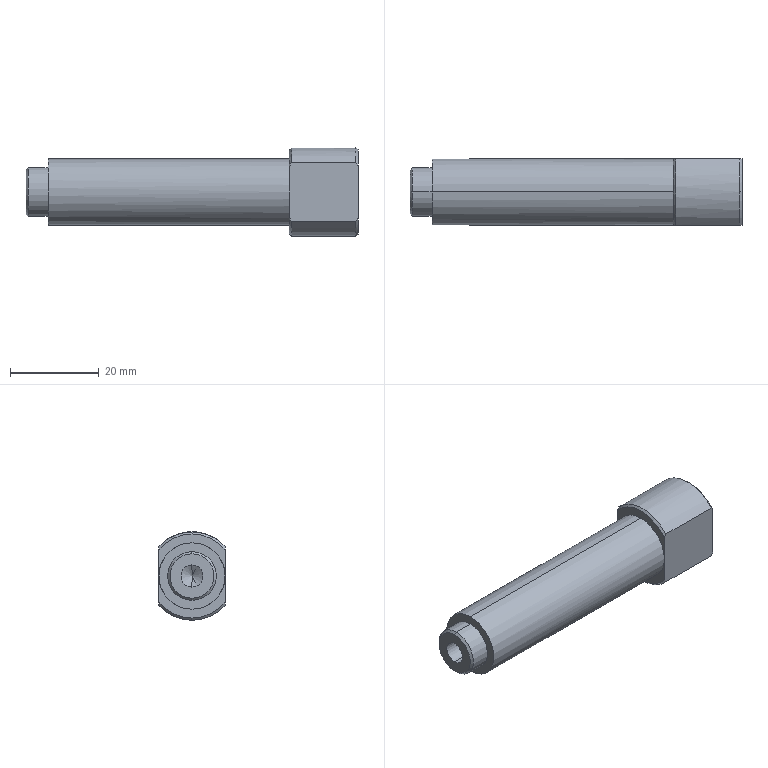Part | SolidWorks | features Chamfer 3, ICE 3, HoleWzd 1, Revolution 1 | 1 solid | 26 faces | box 75 x 15 x 20 mm | volume 13956 mm3 | cone 10 | cylinder 9 | plane 7 | commonest cylinder face diameters 20 x3 5 x2 11 x2 15 x2
STEP:
#1=CARTESIAN_POINT('',(-37.5,0.,5.));
#2=VERTEX_POINT('',#1);
#3=CARTESIAN_POINT('',(-37.5,0.,-5.));
#4=VERTEX_POINT('',#3);
#5=CARTESIAN_POINT('',(-37.5,0.,0.));
#6=DIRECTION('',(-1.,0.,0.));
#7=DIRECTION('',(0.,0.,-1.));
#8=AXIS2_PLACEMENT_3D('',#5,#6,#7);
#9=CIRCLE('',#8,5.);
#10=EDGE_CURVE('',#2,#4,#9,.T.);
#11=ORIENTED_EDGE('',*,*,#10,.F.);
#12=CARTESIAN_POINT('',(-37.,0.,5.5));
#13=VERTEX_POINT('',#12);
#14=CARTESIAN_POINT('',(-37.5,0.,5.));
#15=DIRECTION('',(0.7071,0.,0.7071));
#16=VECTOR('',#15,1000.);
#17=LINE('',#14,#16);
#18=EDGE_CURVE('',#2,#13,#17,.T.);
#19=ORIENTED_EDGE('',*,*,#18,.T.);
#20=CARTESIAN_POINT('',(-37.,0.,-5.5));
#21=VERTEX_POINT('',#20);
#22=CARTESIAN_POINT('',(-37.,0.,0.));
#23=DIRECTION('',(1.,0.,0.));
#24=DIRECTION('',(0.,0.,-1.));
#25=AXIS2_PLACEMENT_3D('',#22,#23,#24);
#26=CIRCLE('',#25,5.5);
#27=EDGE_CURVE('',#21,#13,#26,.T.);
#28=ORIENTED_EDGE('',*,*,#27,.F.);
#29=CARTESIAN_POINT('',(-37.5,0.,-5.));
#30=DIRECTION('',(0.7071,0.,-0.7071));
#31=VECTOR('',#30,1000.);
#32=LINE('',#29,#31);
#33=EDGE_CURVE('',#4,#21,#32,.T.);
#34=ORIENTED_EDGE('',*,*,#33,.F.);
#35=EDGE_LOOP('',(#11,#19,#28,#34));
#36=FACE_OUTER_BOUND('',#35,.T.);
#37=CARTESIAN_POINT('',(-37.5,0.,0.));
#38=DIRECTION('',(1.,0.,0.));
#39=DIRECTION('',(0.,0.,-1.));
#40=AXIS2_PLACEMENT_3D('',#37,#38,#39);
#41=CONICAL_SURFACE('',#40,5.,0.7854);
#42=ADVANCED_FACE('',(#36),#41,.T.);
#43=CARTESIAN_POINT('',(-22.5,0.,-2.5));
#44=VERTEX_POINT('',#43);
#45=CARTESIAN_POINT('',(-22.5,0.,2.5));
#46=VERTEX_POINT('',#45);
#47=CARTESIAN_POINT('',(-22.5,0.,0.));
#48=DIRECTION('',(-1.,0.,0.));
#49=DIRECTION('',(0.,0.,1.));
#50=AXIS2_PLACEMENT_3D('',#47,#48,#49);
#51=CIRCLE('',#50,2.5);
#52=EDGE_CURVE('',#44,#46,#51,.T.);
#53=ORIENTED_EDGE('',*,*,#52,.F.);
#54=CARTESIAN_POINT('',(-37.5,0.,-2.5));
#55=VERTEX_POINT('',#54);
#56=CARTESIAN_POINT('',(-37.5,0.,-2.5));
#57=DIRECTION('',(-1.,0.,0.));
#58=VECTOR('',#57,1000.);
#59=LINE('',#56,#58);
#60=EDGE_CURVE('',#44,#55,#59,.T.);
#61=ORIENTED_EDGE('',*,*,#60,.T.);
#62=CARTESIAN_POINT('',(-37.5,0.,2.5));
#63=VERTEX_POINT('',#62);
#64=CARTESIAN_POINT('',(-37.5,0.,0.));
#65=DIRECTION('',(-1.,0.,0.));
#66=DIRECTION('',(0.,0.,1.));
#67=AXIS2_PLACEMENT_3D('',#64,#65,#66);
#68=CIRCLE('',#67,2.5);
#69=EDGE_CURVE('',#55,#63,#68,.T.);
#70=ORIENTED_EDGE('',*,*,#69,.T.);
#71=CARTESIAN_POINT('',(-37.5,0.,2.5));
#72=DIRECTION('',(-1.,0.,0.));
#73=VECTOR('',#72,1000.);
#74=LINE('',#71,#73);
#75=EDGE_CURVE('',#46,#63,#74,.T.);
#76=ORIENTED_EDGE('',*,*,#75,.F.);
#77=EDGE_LOOP('',(#53,#61,#70,#76));
#78=FACE_OUTER_BOUND('',#77,.T.);
#79=CARTESIAN_POINT('',(-37.5,0.,0.));
#80=DIRECTION('',(-1.,0.,0.));
#81=DIRECTION('',(0.,0.,1.));
#82=AXIS2_PLACEMENT_3D('',#79,#80,#81);
#83=CYLINDRICAL_SURFACE('',#82,2.5);
#84=ADVANCED_FACE('',(#78),#83,.F.);
#85=CARTESIAN_POINT('',(-20.998,0.,0.));
#86=VERTEX_POINT('',#85);
#87=CARTESIAN_POINT('',(-22.5,0.,2.5));
#88=DIRECTION('',(-0.515,0.,0.8572));
#89=VECTOR('',#88,1000.);
#90=LINE('',#87,#89);
#91=EDGE_CURVE('',#86,#46,#90,.T.);
#92=ORIENTED_EDGE('',*,*,#91,.F.);
#93=CARTESIAN_POINT('',(-22.5,0.,-2.5));
#94=DIRECTION('',(-0.515,0.,-0.8572));
#95=VECTOR('',#94,1000.);
#96=LINE('',#93,#95);
#97=EDGE_CURVE('',#86,#44,#96,.T.);
#98=ORIENTED_EDGE('',*,*,#97,.T.);
#99=ORIENTED_EDGE('',*,*,#52,.T.);
#100=EDGE_LOOP('',(#92,#98,#99));
#101=FACE_OUTER_BOUND('',#100,.T.);
#102=CARTESIAN_POINT('',(-22.5,0.,0.));
#103=DIRECTION('',(-1.,0.,0.));
#104=DIRECTION('',(0.,0.,1.));
#105=AXIS2_PLACEMENT_3D('',#102,#103,#104);
#106=CONICAL_SURFACE('',#105,2.5,1.03);
#107=ADVANCED_FACE('',(#101),#106,.F.);
#108=CARTESIAN_POINT('',(-32.5,0.,5.5));
#109=VERTEX_POINT('',#108);
#110=CARTESIAN_POINT('',(-32.5,0.,-5.5));
#111=VERTEX_POINT('',#110);
#112=CARTESIAN_POINT('',(-32.5,0.,0.));
#113=DIRECTION('',(-1.,0.,0.));
#114=DIRECTION('',(0.,0.,1.));
#115=AXIS2_PLACEMENT_3D('',#112,#113,#114);
#116=CIRCLE('',#115,5.5);
#117=EDGE_CURVE('',#109,#111,#116,.T.);
#118=ORIENTED_EDGE('',*,*,#117,.T.);
#119=CARTESIAN_POINT('',(-32.5,0.,-5.5));
#120=DIRECTION('',(-1.,0.,0.));
#121=VECTOR('',#120,1000.);
#122=LINE('',#119,#121);
#123=EDGE_CURVE('',#111,#21,#122,.T.);
#124=ORIENTED_EDGE('',*,*,#123,.T.);
#125=ORIENTED_EDGE('',*,*,#27,.T.);
#126=CARTESIAN_POINT('',(-32.5,0.,5.5));
#127=DIRECTION('',(-1.,0.,0.));
#128=VECTOR('',#127,1000.);
#129=LINE('',#126,#128);
#130=EDGE_CURVE('',#109,#13,#129,.T.);
#131=ORIENTED_EDGE('',*,*,#130,.F.);
#132=EDGE_LOOP('',(#118,#124,#125,#131));
#133=FACE_OUTER_BOUND('',#132,.T.);
#134=CARTESIAN_POINT('',(-32.5,0.,0.));
#135=DIRECTION('',(-1.,0.,0.));
#136=DIRECTION('',(0.,0.,1.));
#137=AXIS2_PLACEMENT_3D('',#134,#135,#136);
#138=CYLINDRICAL_SURFACE('',#137,5.5);
#139=ADVANCED_FACE('',(#133),#138,.T.);
#140=CARTESIAN_POINT('',(37.5,0.,9.5));
#141=VERTEX_POINT('',#140);
#142=CARTESIAN_POINT('',(37.5,-7.5,5.831));
#143=VERTEX_POINT('',#142);
#144=CARTESIAN_POINT('',(37.5,0.,0.));
#145=DIRECTION('',(1.,0.,0.));
#146=DIRECTION('',(0.,0.,1.));
#147=AXIS2_PLACEMENT_3D('',#144,#145,#146);
#148=CIRCLE('',#147,9.5);
#149=EDGE_CURVE('',#141,#143,#148,.T.);
#150=ORIENTED_EDGE('',*,*,#149,.F.);
#151=CARTESIAN_POINT('',(37.,0.,10.));
#152=VERTEX_POINT('',#151);
#153=CARTESIAN_POINT('',(37.5,0.,9.5));
#154=DIRECTION('',(-0.7071,0.,0.7071));
#155=VECTOR('',#154,1000.);
#156=LINE('',#153,#155);
#157=EDGE_CURVE('',#141,#152,#156,.T.);
#158=ORIENTED_EDGE('',*,*,#157,.T.);
#159=CARTESIAN_POINT('',(37.,-7.5,6.614));
#160=VERTEX_POINT('',#159);
#161=CARTESIAN_POINT('',(37.,0.,0.));
#162=DIRECTION('',(-1.,0.,0.));
#163=DIRECTION('',(0.,0.,1.));
#164=AXIS2_PLACEMENT_3D('',#161,#162,#163);
#165=CIRCLE('',#164,10.);
#166=EDGE_CURVE('',#160,#152,#165,.T.);
#167=ORIENTED_EDGE('',*,*,#166,.F.);
#168=CARTESIAN_POINT('',(37.,-7.5,6.614));
#169=CARTESIAN_POINT('',(37.171,-7.5,6.356));
#170=CARTESIAN_POINT('',(37.338,-7.5,6.095));
#171=CARTESIAN_POINT('',(37.5,-7.5,5.831));
#172=B_SPLINE_CURVE_WITH_KNOTS('',3,(#168,#169,#170,#171),.UNSPECIFIED.,.F.,.F.,(4,4),(0.00000126,0.000926),.UNSPECIFIED.);
#173=EDGE_CURVE('',#160,#143,#172,.T.);
#174=ORIENTED_EDGE('',*,*,#173,.T.);
#175=EDGE_LOOP('',(#150,#158,#167,#174));
#176=FACE_OUTER_BOUND('',#175,.T.);
#177=CARTESIAN_POINT('',(37.5,0.,0.));
#178=DIRECTION('',(-1.,0.,0.));
#179=DIRECTION('',(0.,0.,1.));
#180=AXIS2_PLACEMENT_3D('',#177,#178,#179);
#181=CONICAL_SURFACE('',#180,9.5,0.7854);
#182=ADVANCED_FACE('',(#176),#181,.T.);
#183=CARTESIAN_POINT('',(22.,0.,-9.5));
#184=VERTEX_POINT('',#183);
#185=CARTESIAN_POINT('',(22.,-7.5,-5.831));
#186=VERTEX_POINT('',#185);
#187=CARTESIAN_POINT('',(22.,0.,0.));
#188=DIRECTION('',(-1.,0.,0.));
#189=DIRECTION('',(0.,0.,-1.));
#190=AXIS2_PLACEMENT_3D('',#187,#188,#189);
#191=CIRCLE('',#190,9.5);
#192=EDGE_CURVE('',#184,#186,#191,.T.);
#193=ORIENTED_EDGE('',*,*,#192,.F.);
#194=CARTESIAN_POINT('',(22.5,0.,-10.));
#195=VERTEX_POINT('',#194);
#196=CARTESIAN_POINT('',(22.5,0.,-10.));
#197=DIRECTION('',(0.7071,0.,-0.7071));
#198=VECTOR('',#197,1000.);
#199=LINE('',#196,#198);
#200=EDGE_CURVE('',#184,#195,#199,.T.);
#201=ORIENTED_EDGE('',*,*,#200,.T.);
#202=CARTESIAN_POINT('',(22.5,-7.5,-6.614));
#203=VERTEX_POINT('',#202);
#204=CARTESIAN_POINT('',(22.5,0.,0.));
#205=DIRECTION('',(1.,0.,0.));
#206=DIRECTION('',(0.,0.,-1.));
#207=AXIS2_PLACEMENT_3D('',#204,#205,#206);
#208=CIRCLE('',#207,10.);
#209=EDGE_CURVE('',#203,#195,#208,.T.);
#210=ORIENTED_EDGE('',*,*,#209,.F.);
#211=CARTESIAN_POINT('',(22.5,-7.5,-6.614));
#212=CARTESIAN_POINT('',(22.329,-7.5,-6.356));
#213=CARTESIAN_POINT('',(22.162,-7.5,-6.095));
#214=CARTESIAN_POINT('',(22.,-7.5,-5.831));
#215=B_SPLINE_CURVE_WITH_KNOTS('',3,(#211,#212,#213,#214),.UNSPECIFIED.,.F.,.F.,(4,4),(0.00000126,0.000926),.UNSPECIFIED.);
#216=EDGE_CURVE('',#203,#186,#215,.T.);
#217=ORIENTED_EDGE('',*,*,#216,.T.);
#218=EDGE_LOOP('',(#193,#201,#210,#217));
#219=FACE_OUTER_BOUND('',#218,.T.);
#220=CARTESIAN_POINT('',(22.5,0.,0.));
#221=DIRECTION('',(1.,0.,0.));
#222=DIRECTION('',(0.,0.,-1.));
#223=AXIS2_PLACEMENT_3D('',#220,#221,#222);
#224=CONICAL_SURFACE('',#223,10.,0.7854);
#225=ADVANCED_FACE('',(#219),#224,.T.);
#226=ORIENTED_EDGE('',*,*,#209,.T.);
#227=CARTESIAN_POINT('',(37.,0.,-10.));
#228=VERTEX_POINT('',#227);
#229=CARTESIAN_POINT('',(22.,0.,-10.));
#230=DIRECTION('',(1.,0.,0.));
#231=VECTOR('',#230,1000.);
#232=LINE('',#229,#231);
#233=EDGE_CURVE('',#195,#228,#232,.T.);
#234=ORIENTED_EDGE('',*,*,#233,.T.);
#235=CARTESIAN_POINT('',(37.,-7.5,-6.614));
#236=VERTEX_POINT('',#235);
#237=CARTESIAN_POINT('',(37.,0.,0.));
#238=DIRECTION('',(-1.,0.,0.));
#239=DIRECTION('',(0.,0.,1.));
#240=AXIS2_PLACEMENT_3D('',#237,#238,#239);
#241=CIRCLE('',#240,10.);
#242=EDGE_CURVE('',#228,#236,#241,.T.);
#243=ORIENTED_EDGE('',*,*,#242,.T.);
#244=CARTESIAN_POINT('',(22.,-7.5,-6.614));
#245=DIRECTION('',(-1.,0.,0.));
#246=VECTOR('',#245,1000.);
#247=LINE('',#244,#246);
#248=EDGE_CURVE('',#236,#203,#247,.T.);
#249=ORIENTED_EDGE('',*,*,#248,.T.);
#250=EDGE_LOOP('',(#226,#234,#243,#249));
#251=FACE_OUTER_BOUND('',#250,.T.);
#252=CARTESIAN_POINT('',(22.,0.,0.));
#253=DIRECTION('',(1.,0.,0.));
#254=DIRECTION('',(0.,0.,-1.));
#255=AXIS2_PLACEMENT_3D('',#252,#253,#254);
#256=CYLINDRICAL_SURFACE('',#255,10.);
#257=ADVANCED_FACE('',(#251),#256,.T.);
#258=CARTESIAN_POINT('',(22.,0.,-7.5));
#259=VERTEX_POINT('',#258);
#260=CARTESIAN_POINT('',(22.,7.5,0.));
#261=VERTEX_POINT('',#260);
#262=CARTESIAN_POINT('',(22.,0.,0.));
#263=DIRECTION('',(1.,0.,0.));
#264=DIRECTION('',(0.,0.,-1.));
#265=AXIS2_PLACEMENT_3D('',#262,#263,#264);
#266=CIRCLE('',#265,7.5);
#267=EDGE_CURVE('',#259,#261,#266,.T.);
#268=ORIENTED_EDGE('',*,*,#267,.F.);
#269=CARTESIAN_POINT('',(-32.5,0.,-7.5));
#270=VERTEX_POINT('',#269);
#271=CARTESIAN_POINT('',(-37.5,0.,-7.5));
#272=DIRECTION('',(-1.,0.,0.));
#273=VECTOR('',#272,1000.);
#274=LINE('',#271,#273);
#275=EDGE_CURVE('',#259,#270,#274,.T.);
#276=ORIENTED_EDGE('',*,*,#275,.T.);
#277=CARTESIAN_POINT('',(-32.5,0.,7.5));
#278=VERTEX_POINT('',#277);
#279=CARTESIAN_POINT('',(-32.5,0.,0.));
#280=DIRECTION('',(-1.,0.,0.));
#281=DIRECTION('',(0.,0.,1.));
#282=AXIS2_PLACEMENT_3D('',#279,#280,#281);
#283=CIRCLE('',#282,7.5);
#284=EDGE_CURVE('',#278,#270,#283,.T.);
#285=ORIENTED_EDGE('',*,*,#284,.F.);
#286=CARTESIAN_POINT('',(22.,0.,7.5));
#287=VERTEX_POINT('',#286);
#288=CARTESIAN_POINT('',(-37.5,0.,7.5));
#289=DIRECTION('',(-1.,0.,0.));
#290=VECTOR('',#289,1000.);
#291=LINE('',#288,#290);
#292=EDGE_CURVE('',#287,#278,#291,.T.);
#293=ORIENTED_EDGE('',*,*,#292,.F.);
#294=CARTESIAN_POINT('',(22.,0.,0.));
#295=DIRECTION('',(1.,0.,0.));
#296=DIRECTION('',(0.,0.,-1.));
#297=AXIS2_PLACEMENT_3D('',#294,#295,#296);
#298=CIRCLE('',#297,7.5);
#299=EDGE_CURVE('',#261,#287,#298,.T.);
#300=ORIENTED_EDGE('',*,*,#299,.F.);
#301=EDGE_LOOP('',(#268,#276,#285,#293,#300));
#302=FACE_OUTER_BOUND('',#301,.T.);
#303=CARTESIAN_POINT('',(-37.5,0.,0.));
#304=DIRECTION('',(-1.,0.,0.));
#305=DIRECTION('',(0.,0.,1.));
#306=AXIS2_PLACEMENT_3D('',#303,#304,#305);
#307=CYLINDRICAL_SURFACE('',#306,7.5);
#308=ADVANCED_FACE('',(#302),#307,.T.);
#309=ORIENTED_EDGE('',*,*,#275,.F.);
#310=CARTESIAN_POINT('',(22.,-7.5,0.));
#311=VERTEX_POINT('',#310);
#312=CARTESIAN_POINT('',(22.,0.,0.));
#313=DIRECTION('',(1.,0.,0.));
#314=DIRECTION('',(0.,0.,-1.));
#315=AXIS2_PLACEMENT_3D('',#312,#313,#314);
#316=CIRCLE('',#315,7.5);
#317=EDGE_CURVE('',#311,#259,#316,.T.);
#318=ORIENTED_EDGE('',*,*,#317,.F.);
#319=CARTESIAN_POINT('',(22.,0.,0.));
#320=DIRECTION('',(1.,0.,0.));
#321=DIRECTION('',(0.,0.,-1.));
#322=AXIS2_PLACEMENT_3D('',#319,#320,#321);
#323=CIRCLE('',#322,7.5);
#324=EDGE_CURVE('',#287,#311,#323,.T.);
#325=ORIENTED_EDGE('',*,*,#324,.F.);
#326=ORIENTED_EDGE('',*,*,#292,.T.);
#327=CARTESIAN_POINT('',(-32.5,0.,0.));
#328=DIRECTION('',(-1.,0.,0.));
#329=DIRECTION('',(0.,0.,1.));
#330=AXIS2_PLACEMENT_3D('',#327,#328,#329);
#331=CIRCLE('',#330,7.5);
#332=EDGE_CURVE('',#270,#278,#331,.T.);
#333=ORIENTED_EDGE('',*,*,#332,.F.);
#334=EDGE_LOOP('',(#309,#318,#325,#326,#333));
#335=FACE_OUTER_BOUND('',#334,.T.);
#336=CARTESIAN_POINT('',(-37.5,0.,0.));
#337=DIRECTION('',(-1.,0.,0.));
#338=DIRECTION('',(0.,0.,1.));
#339=AXIS2_PLACEMENT_3D('',#336,#337,#338);
#340=CYLINDRICAL_SURFACE('',#339,7.5);
#341=ADVANCED_FACE('',(#335),#340,.T.);
#342=ORIENTED_EDGE('',*,*,#233,.F.);
#343=CARTESIAN_POINT('',(22.5,7.5,-6.614));
#344=VERTEX_POINT('',#343);
#345=CARTESIAN_POINT('',(22.5,0.,0.));
#346=DIRECTION('',(1.,0.,0.));
#347=DIRECTION('',(0.,0.,-1.));
#348=AXIS2_PLACEMENT_3D('',#345,#346,#347);
#349=CIRCLE('',#348,10.);
#350=EDGE_CURVE('',#195,#344,#349,.T.);
#351=ORIENTED_EDGE('',*,*,#350,.T.);
#352=CARTESIAN_POINT('',(37.,7.5,-6.614));
#353=VERTEX_POINT('',#352);
#354=CARTESIAN_POINT('',(22.,7.5,-6.614));
#355=DIRECTION('',(1.,0.,0.));
#356=VECTOR('',#355,1000.);
#357=LINE('',#354,#356);
#358=EDGE_CURVE('',#344,#353,#357,.T.);
#359=ORIENTED_EDGE('',*,*,#358,.T.);
#360=CARTESIAN_POINT('',(37.,0.,0.));
#361=DIRECTION('',(-1.,0.,0.));
#362=DIRECTION('',(0.,0.,1.));
#363=AXIS2_PLACEMENT_3D('',#360,#361,#362);
#364=CIRCLE('',#363,10.);
#365=EDGE_CURVE('',#353,#228,#364,.T.);
#366=ORIENTED_EDGE('',*,*,#365,.T.);
#367=EDGE_LOOP('',(#342,#351,#359,#366));
#368=FACE_OUTER_BOUND('',#367,.T.);
#369=CARTESIAN_POINT('',(22.,0.,0.));
#370=DIRECTION('',(1.,0.,0.));
#371=DIRECTION('',(0.,0.,-1.));
#372=AXIS2_PLACEMENT_3D('',#369,#370,#371);
#373=CYLINDRICAL_SURFACE('',#372,10.);
#374=ADVANCED_FACE('',(#368),#373,.T.);
#375=CARTESIAN_POINT('',(22.5,7.5,6.614));
#376=VERTEX_POINT('',#375);
#377=CARTESIAN_POINT('',(22.5,-7.5,6.614));
#378=VERTEX_POINT('',#377);
#379=CARTESIAN_POINT('',(22.5,0.,0.));
#380=DIRECTION('',(1.,0.,0.));
#381=DIRECTION('',(0.,0.,-1.));
#382=AXIS2_PLACEMENT_3D('',#379,#380,#381);
#383=CIRCLE('',#382,10.);
#384=EDGE_CURVE('',#376,#378,#383,.T.);
#385=ORIENTED_EDGE('',*,*,#384,.T.);
#386=CARTESIAN_POINT('',(22.,-7.5,6.614));
#387=DIRECTION('',(1.,0.,0.));
#388=VECTOR('',#387,1000.);
#389=LINE('',#386,#388);
#390=EDGE_CURVE('',#378,#160,#389,.T.);
#391=ORIENTED_EDGE('',*,*,#390,.T.);
#392=ORIENTED_EDGE('',*,*,#166,.T.);
#393=CARTESIAN_POINT('',(37.,7.5,6.614));
#394=VERTEX_POINT('',#393);
#395=CARTESIAN_POINT('',(37.,0.,0.));
#396=DIRECTION('',(-1.,0.,0.));
#397=DIRECTION('',(0.,0.,1.));
#398=AXIS2_PLACEMENT_3D('',#395,#396,#397);
#399=CIRCLE('',#398,10.);
#400=EDGE_CURVE('',#152,#394,#399,.T.);
#401=ORIENTED_EDGE('',*,*,#400,.T.);
#402=CARTESIAN_POINT('',(22.,7.5,6.614));
#403=DIRECTION('',(-1.,0.,0.));
#404=VECTOR('',#403,1000.);
#405=LINE('',#402,#404);
#406=EDGE_CURVE('',#394,#376,#405,.T.);
#407=ORIENTED_EDGE('',*,*,#406,.T.);
#408=EDGE_LOOP('',(#385,#391,#392,#401,#407));
#409=FACE_OUTER_BOUND('',#408,.T.);
#410=CARTESIAN_POINT('',(22.,0.,0.));
#411=DIRECTION('',(1.,0.,0.));
#412=DIRECTION('',(0.,0.,-1.));
#413=AXIS2_PLACEMENT_3D('',#410,#411,#412);
#414=CYLINDRICAL_SURFACE('',#413,10.);
#415=ADVANCED_FACE('',(#409),#414,.T.);
#416=CARTESIAN_POINT('',(22.,-7.5,5.831));
#417=VERTEX_POINT('',#416);
#418=CARTESIAN_POINT('',(22.,-7.5,-12.5));
#419=DIRECTION('',(0.,0.,1.));
#420=VECTOR('',#419,1000.);
#421=LINE('',#418,#420);
#422=EDGE_CURVE('',#311,#417,#421,.T.);
#423=ORIENTED_EDGE('',*,*,#422,.T.);
#424=CARTESIAN_POINT('',(22.,7.5,5.831));
#425=VERTEX_POINT('',#424);
#426=CARTESIAN_POINT('',(22.,0.,0.));
#427=DIRECTION('',(-1.,0.,0.));
#428=DIRECTION('',(0.,0.,-1.));
#429=AXIS2_PLACEMENT_3D('',#426,#427,#428);
#430=CIRCLE('',#429,9.5);
#431=EDGE_CURVE('',#417,#425,#430,.T.);
#432=ORIENTED_EDGE('',*,*,#431,.T.);
#433=CARTESIAN_POINT('',(22.,7.5,-12.5));
#434=DIRECTION('',(0.,0.,-1.));
#435=VECTOR('',#434,1000.);
#436=LINE('',#433,#435);
#437=EDGE_CURVE('',#425,#261,#436,.T.);
#438=ORIENTED_EDGE('',*,*,#437,.T.);
#439=ORIENTED_EDGE('',*,*,#299,.T.);
#440=ORIENTED_EDGE('',*,*,#324,.T.);
#441=EDGE_LOOP('',(#423,#432,#438,#439,#440));
#442=FACE_OUTER_BOUND('',#441,.T.);
#443=CARTESIAN_POINT('',(22.,0.,0.));
#444=DIRECTION('',(1.,0.,0.));
#445=DIRECTION('',(0.,0.,-1.));
#446=AXIS2_PLACEMENT_3D('',#443,#444,#445);
#447=PLANE('',#446);
#448=ADVANCED_FACE('',(#442),#447,.F.);
#449=CARTESIAN_POINT('',(22.,-7.5,-12.5));
#450=DIRECTION('',(0.,0.,1.));
#451=VECTOR('',#450,1000.);
#452=LINE('',#449,#451);
#453=EDGE_CURVE('',#186,#311,#452,.T.);
#454=ORIENTED_EDGE('',*,*,#453,.T.);
#455=ORIENTED_EDGE('',*,*,#317,.T.);
#456=ORIENTED_EDGE('',*,*,#267,.T.);
#457=CARTESIAN_POINT('',(22.,7.5,-5.831));
#458=VERTEX_POINT('',#457);
#459=CARTESIAN_POINT('',(22.,7.5,-12.5));
#460=DIRECTION('',(0.,0.,-1.));
#461=VECTOR('',#460,1000.);
#462=LINE('',#459,#461);
#463=EDGE_CURVE('',#261,#458,#462,.T.);
#464=ORIENTED_EDGE('',*,*,#463,.T.);
#465=CARTESIAN_POINT('',(22.,0.,0.));
#466=DIRECTION('',(-1.,0.,0.));
#467=DIRECTION('',(0.,0.,-1.));
#468=AXIS2_PLACEMENT_3D('',#465,#466,#467);
#469=CIRCLE('',#468,9.5);
#470=EDGE_CURVE('',#458,#184,#469,.T.);
#471=ORIENTED_EDGE('',*,*,#470,.T.);
#472=ORIENTED_EDGE('',*,*,#192,.T.);
#473=EDGE_LOOP('',(#454,#455,#456,#464,#471,#472));
#474=FACE_OUTER_BOUND('',#473,.T.);
#475=CARTESIAN_POINT('',(22.,0.,0.));
#476=DIRECTION('',(1.,0.,0.));
#477=DIRECTION('',(0.,0.,-1.));
#478=AXIS2_PLACEMENT_3D('',#475,#476,#477);
#479=PLANE('',#478);
#480=ADVANCED_FACE('',(#474),#479,.F.);
#481=CARTESIAN_POINT('',(37.5,-7.5,-5.831));
#482=VERTEX_POINT('',#481);
#483=CARTESIAN_POINT('',(37.5,-7.5,-12.5));
#484=DIRECTION('',(0.,0.,1.));
#485=VECTOR('',#484,1000.);
#486=LINE('',#483,#485);
#487=EDGE_CURVE('',#482,#143,#486,.T.);
#488=ORIENTED_EDGE('',*,*,#487,.F.);
#489=CARTESIAN_POINT('',(37.5,7.5,-5.831));
#490=VERTEX_POINT('',#489);
#491=CARTESIAN_POINT('',(37.5,0.,0.));
#492=DIRECTION('',(1.,0.,0.));
#493=DIRECTION('',(0.,0.,1.));
#494=AXIS2_PLACEMENT_3D('',#491,#492,#493);
#495=CIRCLE('',#494,9.5);
#496=EDGE_CURVE('',#482,#490,#495,.T.);
#497=ORIENTED_EDGE('',*,*,#496,.T.);
#498=CARTESIAN_POINT('',(37.5,7.5,5.831));
#499=VERTEX_POINT('',#498);
#500=CARTESIAN_POINT('',(37.5,7.5,-12.5));
#501=DIRECTION('',(0.,0.,-1.));
#502=VECTOR('',#501,1000.);
#503=LINE('',#500,#502);
#504=EDGE_CURVE('',#499,#490,#503,.T.);
#505=ORIENTED_EDGE('',*,*,#504,.F.);
#506=CARTESIAN_POINT('',(37.5,0.,0.));
#507=DIRECTION('',(1.,0.,0.));
#508=DIRECTION('',(0.,0.,1.));
#509=AXIS2_PLACEMENT_3D('',#506,#507,#508);
#510=CIRCLE('',#509,9.5);
#511=EDGE_CURVE('',#499,#141,#510,.T.);
#512=ORIENTED_EDGE('',*,*,#511,.T.);
#513=ORIENTED_EDGE('',*,*,#149,.T.);
#514=EDGE_LOOP('',(#488,#497,#505,#512,#513));
#515=FACE_OUTER_BOUND('',#514,.T.);
#516=CARTESIAN_POINT('',(37.5,7.5,0.));
#517=DIRECTION('',(-1.,0.,0.));
#518=DIRECTION('',(0.,0.,1.));
#519=AXIS2_PLACEMENT_3D('',#516,#517,#518);
#520=PLANE('',#519);
#521=ADVANCED_FACE('',(#515),#520,.F.);
#522=ORIENTED_EDGE('',*,*,#200,.F.);
#523=ORIENTED_EDGE('',*,*,#470,.F.);
#524=CARTESIAN_POINT('',(22.,7.5,-5.831));
#525=CARTESIAN_POINT('',(22.162,7.5,-6.095));
#526=CARTESIAN_POINT('',(22.329,7.5,-6.356));
#527=CARTESIAN_POINT('',(22.5,7.5,-6.614));
#528=B_SPLINE_CURVE_WITH_KNOTS('',3,(#524,#525,#526,#527),.UNSPECIFIED.,.F.,.F.,(4,4),(0.01335,0.01427),.UNSPECIFIED.);
#529=EDGE_CURVE('',#458,#344,#528,.T.);
#530=ORIENTED_EDGE('',*,*,#529,.T.);
#531=ORIENTED_EDGE('',*,*,#350,.F.);
#532=EDGE_LOOP('',(#522,#523,#530,#531));
#533=FACE_OUTER_BOUND('',#532,.T.);
#534=CARTESIAN_POINT('',(22.5,0.,0.));
#535=DIRECTION('',(1.,0.,0.));
#536=DIRECTION('',(0.,0.,-1.));
#537=AXIS2_PLACEMENT_3D('',#534,#535,#536);
#538=CONICAL_SURFACE('',#537,10.,0.7854);
#539=ADVANCED_FACE('',(#533),#538,.T.);
#540=ORIENTED_EDGE('',*,*,#431,.F.);
#541=CARTESIAN_POINT('',(22.,-7.5,5.831));
#542=CARTESIAN_POINT('',(22.162,-7.5,6.095));
#543=CARTESIAN_POINT('',(22.329,-7.5,6.356));
#544=CARTESIAN_POINT('',(22.5,-7.5,6.614));
#545=B_SPLINE_CURVE_WITH_KNOTS('',3,(#541,#542,#543,#544),.UNSPECIFIED.,.F.,.F.,(4,4),(0.01335,0.01427),.UNSPECIFIED.);
#546=EDGE_CURVE('',#417,#378,#545,.T.);
#547=ORIENTED_EDGE('',*,*,#546,.T.);
#548=ORIENTED_EDGE('',*,*,#384,.F.);
#549=CARTESIAN_POINT('',(22.5,7.5,6.614));
#550=CARTESIAN_POINT('',(22.329,7.5,6.356));
#551=CARTESIAN_POINT('',(22.162,7.5,6.095));
#552=CARTESIAN_POINT('',(22.,7.5,5.831));
#553=B_SPLINE_CURVE_WITH_KNOTS('',3,(#549,#550,#551,#552),.UNSPECIFIED.,.F.,.F.,(4,4),(0.00000126,0.000926),.UNSPECIFIED.);
#554=EDGE_CURVE('',#376,#425,#553,.T.);
#555=ORIENTED_EDGE('',*,*,#554,.T.);
#556=EDGE_LOOP('',(#540,#547,#548,#555));
#557=FACE_OUTER_BOUND('',#556,.T.);
#558=CARTESIAN_POINT('',(22.5,0.,0.));
#559=DIRECTION('',(1.,0.,0.));
#560=DIRECTION('',(0.,0.,-1.));
#561=AXIS2_PLACEMENT_3D('',#558,#559,#560);
#562=CONICAL_SURFACE('',#561,10.,0.7854);
#563=ADVANCED_FACE('',(#557),#562,.T.);
#564=ORIENTED_EDGE('',*,*,#157,.F.);
#565=ORIENTED_EDGE('',*,*,#511,.F.);
#566=CARTESIAN_POINT('',(37.5,7.5,5.831));
#567=CARTESIAN_POINT('',(37.338,7.5,6.095));
#568=CARTESIAN_POINT('',(37.171,7.5,6.356));
#569=CARTESIAN_POINT('',(37.,7.5,6.614));
#570=B_SPLINE_CURVE_WITH_KNOTS('',3,(#566,#567,#568,#569),.UNSPECIFIED.,.F.,.F.,(4,4),(0.01335,0.01427),.UNSPECIFIED.);
#571=EDGE_CURVE('',#499,#394,#570,.T.);
#572=ORIENTED_EDGE('',*,*,#571,.T.);
#573=ORIENTED_EDGE('',*,*,#400,.F.);
#574=EDGE_LOOP('',(#564,#565,#572,#573));
#575=FACE_OUTER_BOUND('',#574,.T.);
#576=CARTESIAN_POINT('',(37.5,0.,0.));
#577=DIRECTION('',(-1.,0.,0.));
#578=DIRECTION('',(0.,0.,1.));
#579=AXIS2_PLACEMENT_3D('',#576,#577,#578);
#580=CONICAL_SURFACE('',#579,9.5,0.7854);
#581=ADVANCED_FACE('',(#575),#580,.T.);
#582=ORIENTED_EDGE('',*,*,#496,.F.);
#583=CARTESIAN_POINT('',(37.5,-7.5,-5.831));
#584=CARTESIAN_POINT('',(37.338,-7.5,-6.095));
#585=CARTESIAN_POINT('',(37.171,-7.5,-6.356));
#586=CARTESIAN_POINT('',(37.,-7.5,-6.614));
#587=B_SPLINE_CURVE_WITH_KNOTS('',3,(#583,#584,#585,#586),.UNSPECIFIED.,.F.,.F.,(4,4),(0.01335,0.01427),.UNSPECIFIED.);
#588=EDGE_CURVE('',#482,#236,#587,.T.);
#589=ORIENTED_EDGE('',*,*,#588,.T.);
#590=ORIENTED_EDGE('',*,*,#242,.F.);
#591=ORIENTED_EDGE('',*,*,#365,.F.);
#592=CARTESIAN_POINT('',(37.,7.5,-6.614));
#593=CARTESIAN_POINT('',(37.171,7.5,-6.356));
#594=CARTESIAN_POINT('',(37.338,7.5,-6.095));
#595=CARTESIAN_POINT('',(37.5,7.5,-5.831));
#596=B_SPLINE_CURVE_WITH_KNOTS('',3,(#592,#593,#594,#595),.UNSPECIFIED.,.F.,.F.,(4,4),(0.00000126,0.000926),.UNSPECIFIED.);
#597=EDGE_CURVE('',#353,#490,#596,.T.);
#598=ORIENTED_EDGE('',*,*,#597,.T.);
#599=EDGE_LOOP('',(#582,#589,#590,#591,#598));
#600=FACE_OUTER_BOUND('',#599,.T.);
#601=CARTESIAN_POINT('',(37.5,0.,0.));
#602=DIRECTION('',(-1.,0.,0.));
#603=DIRECTION('',(0.,0.,1.));
#604=AXIS2_PLACEMENT_3D('',#601,#602,#603);
#605=CONICAL_SURFACE('',#604,9.5,0.7854);
#606=ADVANCED_FACE('',(#600),#605,.T.);
#607=ORIENTED_EDGE('',*,*,#463,.F.);
#608=ORIENTED_EDGE('',*,*,#437,.F.);
#609=ORIENTED_EDGE('',*,*,#554,.F.);
#610=ORIENTED_EDGE('',*,*,#406,.F.);
#611=ORIENTED_EDGE('',*,*,#571,.F.);
#612=ORIENTED_EDGE('',*,*,#504,.T.);
#613=ORIENTED_EDGE('',*,*,#597,.F.);
#614=ORIENTED_EDGE('',*,*,#358,.F.);
#615=ORIENTED_EDGE('',*,*,#529,.F.);
#616=EDGE_LOOP('',(#607,#608,#609,#610,#611,#612,#613,#614,#615));
#617=FACE_OUTER_BOUND('',#616,.T.);
#618=CARTESIAN_POINT('',(37.5,7.5,-12.5));
#619=DIRECTION('',(0.,1.,0.));
#620=DIRECTION('',(0.,0.,1.));
#621=AXIS2_PLACEMENT_3D('',#618,#619,#620);
#622=PLANE('',#621);
#623=ADVANCED_FACE('',(#617),#622,.T.);
#624=ORIENTED_EDGE('',*,*,#422,.F.);
#625=ORIENTED_EDGE('',*,*,#453,.F.);
#626=ORIENTED_EDGE('',*,*,#216,.F.);
#627=ORIENTED_EDGE('',*,*,#248,.F.);
#628=ORIENTED_EDGE('',*,*,#588,.F.);
#629=ORIENTED_EDGE('',*,*,#487,.T.);
#630=ORIENTED_EDGE('',*,*,#173,.F.);
#631=ORIENTED_EDGE('',*,*,#390,.F.);
#632=ORIENTED_EDGE('',*,*,#546,.F.);
#633=EDGE_LOOP('',(#624,#625,#626,#627,#628,#629,#630,#631,#632));
#634=FACE_OUTER_BOUND('',#633,.T.);
#635=CARTESIAN_POINT('',(37.5,-7.5,-12.5));
#636=DIRECTION('',(0.,-1.,0.));
#637=DIRECTION('',(0.,0.,-1.));
#638=AXIS2_PLACEMENT_3D('',#635,#636,#637);
#639=PLANE('',#638);
#640=ADVANCED_FACE('',(#634),#639,.T.);
#641=ORIENTED_EDGE('',*,*,#117,.F.);
#642=CARTESIAN_POINT('',(-32.5,0.,0.));
#643=DIRECTION('',(-1.,0.,0.));
#644=DIRECTION('',(0.,0.,1.));
#645=AXIS2_PLACEMENT_3D('',#642,#643,#644);
#646=CIRCLE('',#645,5.5);
#647=EDGE_CURVE('',#111,#109,#646,.T.);
#648=ORIENTED_EDGE('',*,*,#647,.F.);
#649=EDGE_LOOP('',(#641,#648));
#650=FACE_BOUND('',#649,.T.);
#651=ORIENTED_EDGE('',*,*,#284,.T.);
#652=ORIENTED_EDGE('',*,*,#332,.T.);
#653=EDGE_LOOP('',(#651,#652));
#654=FACE_OUTER_BOUND('',#653,.T.);
#655=CARTESIAN_POINT('',(-32.5,0.,0.));
#656=DIRECTION('',(-1.,0.,0.));
#657=DIRECTION('',(0.,0.,1.));
#658=AXIS2_PLACEMENT_3D('',#655,#656,#657);
#659=PLANE('',#658);
#660=ADVANCED_FACE('',(#650,#654),#659,.T.);
#661=ORIENTED_EDGE('',*,*,#123,.F.);
#662=ORIENTED_EDGE('',*,*,#647,.T.);
#663=ORIENTED_EDGE('',*,*,#130,.T.);
#664=CARTESIAN_POINT('',(-37.,0.,0.));
#665=DIRECTION('',(1.,0.,0.));
#666=DIRECTION('',(0.,0.,-1.));
#667=AXIS2_PLACEMENT_3D('',#664,#665,#666);
#668=CIRCLE('',#667,5.5);
#669=EDGE_CURVE('',#13,#21,#668,.T.);
#670=ORIENTED_EDGE('',*,*,#669,.T.);
#671=EDGE_LOOP('',(#661,#662,#663,#670));
#672=FACE_OUTER_BOUND('',#671,.T.);
#673=CARTESIAN_POINT('',(-32.5,0.,0.));
#674=DIRECTION('',(-1.,0.,0.));
#675=DIRECTION('',(0.,0.,1.));
#676=AXIS2_PLACEMENT_3D('',#673,#674,#675);
#677=CYLINDRICAL_SURFACE('',#676,5.5);
#678=ADVANCED_FACE('',(#672),#677,.T.);
#679=ORIENTED_EDGE('',*,*,#97,.F.);
#680=ORIENTED_EDGE('',*,*,#91,.T.);
#681=CARTESIAN_POINT('',(-22.5,0.,0.));
#682=DIRECTION('',(-1.,0.,0.));
#683=DIRECTION('',(0.,0.,1.));
#684=AXIS2_PLACEMENT_3D('',#681,#682,#683);
#685=CIRCLE('',#684,2.5);
#686=EDGE_CURVE('',#46,#44,#685,.T.);
#687=ORIENTED_EDGE('',*,*,#686,.T.);
#688=EDGE_LOOP('',(#679,#680,#687));
#689=FACE_OUTER_BOUND('',#688,.T.);
#690=CARTESIAN_POINT('',(-22.5,0.,0.));
#691=DIRECTION('',(-1.,0.,0.));
#692=DIRECTION('',(0.,0.,1.));
#693=AXIS2_PLACEMENT_3D('',#690,#691,#692);
#694=CONICAL_SURFACE('',#693,2.5,1.03);
#695=ADVANCED_FACE('',(#689),#694,.F.);
#696=ORIENTED_EDGE('',*,*,#60,.F.);
#697=ORIENTED_EDGE('',*,*,#686,.F.);
#698=ORIENTED_EDGE('',*,*,#75,.T.);
#699=CARTESIAN_POINT('',(-37.5,0.,0.));
#700=DIRECTION('',(-1.,0.,0.));
#701=DIRECTION('',(0.,0.,1.));
#702=AXIS2_PLACEMENT_3D('',#699,#700,#701);
#703=CIRCLE('',#702,2.5);
#704=EDGE_CURVE('',#63,#55,#703,.T.);
#705=ORIENTED_EDGE('',*,*,#704,.T.);
#706=EDGE_LOOP('',(#696,#697,#698,#705));
#707=FACE_OUTER_BOUND('',#706,.T.);
#708=CARTESIAN_POINT('',(-37.5,0.,0.));
#709=DIRECTION('',(-1.,0.,0.));
#710=DIRECTION('',(0.,0.,1.));
#711=AXIS2_PLACEMENT_3D('',#708,#709,#710);
#712=CYLINDRICAL_SURFACE('',#711,2.5);
#713=ADVANCED_FACE('',(#707),#712,.F.);
#714=CARTESIAN_POINT('',(-37.5,0.,0.));
#715=DIRECTION('',(-1.,0.,0.));
#716=DIRECTION('',(0.,0.,-1.));
#717=AXIS2_PLACEMENT_3D('',#714,#715,#716);
#718=CIRCLE('',#717,5.);
#719=EDGE_CURVE('',#4,#2,#718,.T.);
#720=ORIENTED_EDGE('',*,*,#719,.T.);
#721=ORIENTED_EDGE('',*,*,#10,.T.);
#722=EDGE_LOOP('',(#720,#721));
#723=FACE_OUTER_BOUND('',#722,.T.);
#724=ORIENTED_EDGE('',*,*,#704,.F.);
#725=ORIENTED_EDGE('',*,*,#69,.F.);
#726=EDGE_LOOP('',(#724,#725));
#727=FACE_BOUND('',#726,.T.);
#728=CARTESIAN_POINT('',(-37.5,7.5,0.));
#729=DIRECTION('',(1.,0.,0.));
#730=DIRECTION('',(0.,0.,-1.));
#731=AXIS2_PLACEMENT_3D('',#728,#729,#730);
#732=PLANE('',#731);
#733=ADVANCED_FACE('',(#723,#727),#732,.F.);
#734=ORIENTED_EDGE('',*,*,#18,.F.);
#735=ORIENTED_EDGE('',*,*,#719,.F.);
#736=ORIENTED_EDGE('',*,*,#33,.T.);
#737=ORIENTED_EDGE('',*,*,#669,.F.);
#738=EDGE_LOOP('',(#734,#735,#736,#737));
#739=FACE_OUTER_BOUND('',#738,.T.);
#740=CARTESIAN_POINT('',(-37.5,0.,0.));
#741=DIRECTION('',(1.,0.,0.));
#742=DIRECTION('',(0.,0.,-1.));
#743=AXIS2_PLACEMENT_3D('',#740,#741,#742);
#744=CONICAL_SURFACE('',#743,5.,0.7854);
#745=ADVANCED_FACE('',(#739),#744,.T.);
#746=CLOSED_SHELL('',(#42,#84,#107,#139,#182,#225,#257,#308,#341,#374,#415,#448,#480,#521,#539,#563,#581,#606,#623,#640,#660,#678,#695,#713,#733,#745));
#747=MANIFOLD_SOLID_BREP('',#746);
#748=CARTESIAN_POINT('',(0.,0.,0.));
#749=DIRECTION('',(0.,0.,1.));
#750=DIRECTION('',(1.,0.,0.));
#751=AXIS2_PLACEMENT_3D('',#748,#749,#750);
#752=(LENGTH_UNIT()NAMED_UNIT(*)SI_UNIT(.MILLI.,.METRE.));
#753=UNCERTAINTY_MEASURE_WITH_UNIT(LENGTH_MEASURE(0.00001),#752,'','');
#754=(NAMED_UNIT(*)PLANE_ANGLE_UNIT()SI_UNIT($,.RADIAN.));
#755=(NAMED_UNIT(*)SI_UNIT($,.STERADIAN.)SOLID_ANGLE_UNIT());
#756=(GEOMETRIC_REPRESENTATION_CONTEXT(3)GLOBAL_UNCERTAINTY_ASSIGNED_CONTEXT((#753))GLOBAL_UNIT_ASSIGNED_CONTEXT((#752,#754,#755))REPRESENTATION_CONTEXT('',''));
#757=ADVANCED_BREP_SHAPE_REPRESENTATION('',(#747,#751),#756);